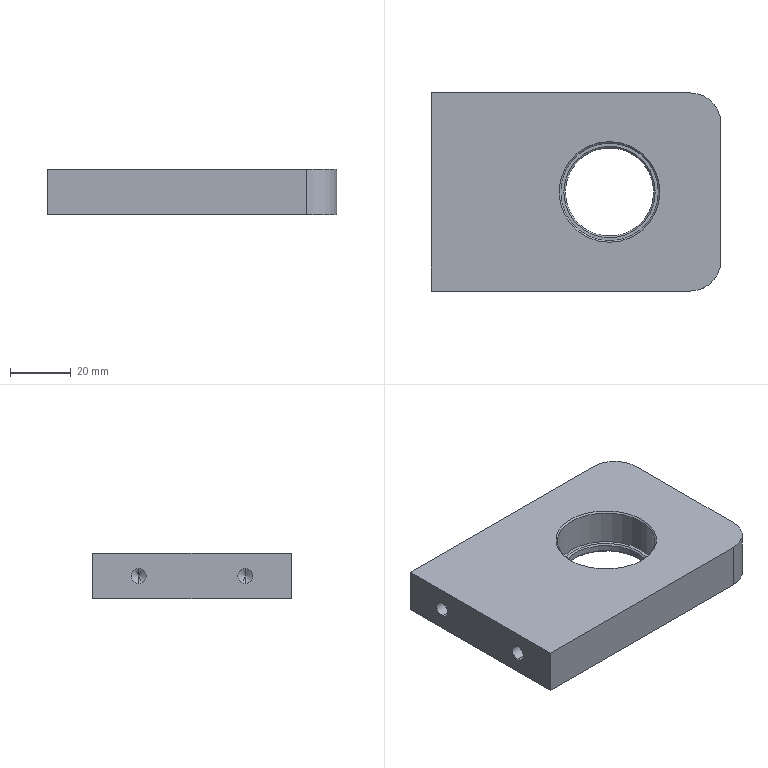Part | STEP file | PN_0012 | 1 solid | 27 faces | box 95 x 65 x 15 mm | volume 79674 mm3 | cylinder 10 | cone 10 | plane 7 | commonest cylinder face diameters 5 x4 20 x2 29 x2 32.05 x2